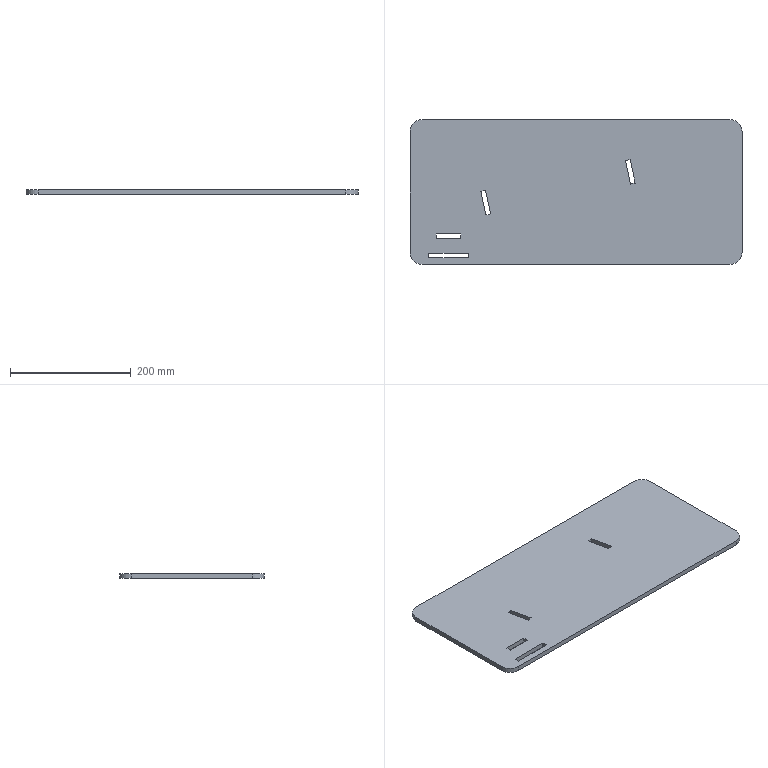Part | SolidWorks | features FlatPattern 1, SMBaseFlange 1, SheetMetal 1 | 1 solid | 26 faces | box 550 x 240 x 8 mm | volume 1041413 mm3 | plane 22 | cylinder 4 | commonest cylinder face diameters 40 x4
STEP:
#1=CARTESIAN_POINT('',(-185.,180.,0.));
#2=VERTEX_POINT('',#1);
#3=CARTESIAN_POINT('',(-205.,160.,0.));
#4=VERTEX_POINT('',#3);
#5=CARTESIAN_POINT('',(-185.,160.,0.));
#6=DIRECTION('',(0.,0.,1.));
#7=DIRECTION('',(1.,0.,0.));
#8=AXIS2_PLACEMENT_3D('',#5,#6,#7);
#9=CIRCLE('',#8,20.);
#10=EDGE_CURVE('',#2,#4,#9,.T.);
#11=ORIENTED_EDGE('',*,*,#10,.F.);
#12=CARTESIAN_POINT('',(-185.,180.,-8.));
#13=VERTEX_POINT('',#12);
#14=CARTESIAN_POINT('',(-185.,180.,-8.));
#15=DIRECTION('',(0.,0.,1.));
#16=VECTOR('',#15,1000.);
#17=LINE('',#14,#16);
#18=EDGE_CURVE('',#13,#2,#17,.T.);
#19=ORIENTED_EDGE('',*,*,#18,.F.);
#20=CARTESIAN_POINT('',(-205.,160.,-8.));
#21=VERTEX_POINT('',#20);
#22=CARTESIAN_POINT('',(-185.,160.,-8.));
#23=DIRECTION('',(0.,0.,1.));
#24=DIRECTION('',(1.,0.,0.));
#25=AXIS2_PLACEMENT_3D('',#22,#23,#24);
#26=CIRCLE('',#25,20.);
#27=EDGE_CURVE('',#13,#21,#26,.T.);
#28=ORIENTED_EDGE('',*,*,#27,.T.);
#29=CARTESIAN_POINT('',(-205.,160.,-8.));
#30=DIRECTION('',(0.,0.,1.));
#31=VECTOR('',#30,1000.);
#32=LINE('',#29,#31);
#33=EDGE_CURVE('',#21,#4,#32,.T.);
#34=ORIENTED_EDGE('',*,*,#33,.T.);
#35=EDGE_LOOP('',(#11,#19,#28,#34));
#36=FACE_OUTER_BOUND('',#35,.T.);
#37=CARTESIAN_POINT('',(-185.,160.,-8.));
#38=DIRECTION('',(0.,0.,1.));
#39=DIRECTION('',(1.,0.,0.));
#40=AXIS2_PLACEMENT_3D('',#37,#38,#39);
#41=CYLINDRICAL_SURFACE('',#40,20.);
#42=ADVANCED_FACE('',(#36),#41,.T.);
#43=CARTESIAN_POINT('',(325.,180.,0.));
#44=VERTEX_POINT('',#43);
#45=CARTESIAN_POINT('',(325.,180.,0.));
#46=DIRECTION('',(-1.,0.,0.));
#47=VECTOR('',#46,1000.);
#48=LINE('',#45,#47);
#49=EDGE_CURVE('',#44,#2,#48,.T.);
#50=ORIENTED_EDGE('',*,*,#49,.F.);
#51=CARTESIAN_POINT('',(325.,180.,-8.));
#52=VERTEX_POINT('',#51);
#53=CARTESIAN_POINT('',(325.,180.,-8.));
#54=DIRECTION('',(0.,0.,1.));
#55=VECTOR('',#54,1000.);
#56=LINE('',#53,#55);
#57=EDGE_CURVE('',#52,#44,#56,.T.);
#58=ORIENTED_EDGE('',*,*,#57,.F.);
#59=CARTESIAN_POINT('',(325.,180.,-8.));
#60=DIRECTION('',(-1.,0.,0.));
#61=VECTOR('',#60,1000.);
#62=LINE('',#59,#61);
#63=EDGE_CURVE('',#52,#13,#62,.T.);
#64=ORIENTED_EDGE('',*,*,#63,.T.);
#65=ORIENTED_EDGE('',*,*,#18,.T.);
#66=EDGE_LOOP('',(#50,#58,#64,#65));
#67=FACE_OUTER_BOUND('',#66,.T.);
#68=CARTESIAN_POINT('',(325.,180.,-8.));
#69=DIRECTION('',(0.,1.,0.));
#70=DIRECTION('',(-1.,0.,0.));
#71=AXIS2_PLACEMENT_3D('',#68,#69,#70);
#72=PLANE('',#71);
#73=ADVANCED_FACE('',(#67),#72,.T.);
#74=CARTESIAN_POINT('',(345.,160.,0.));
#75=VERTEX_POINT('',#74);
#76=CARTESIAN_POINT('',(325.,160.,0.));
#77=DIRECTION('',(0.,0.,1.));
#78=DIRECTION('',(1.,0.,0.));
#79=AXIS2_PLACEMENT_3D('',#76,#77,#78);
#80=CIRCLE('',#79,20.);
#81=EDGE_CURVE('',#75,#44,#80,.T.);
#82=ORIENTED_EDGE('',*,*,#81,.F.);
#83=CARTESIAN_POINT('',(345.,160.,-8.));
#84=VERTEX_POINT('',#83);
#85=CARTESIAN_POINT('',(345.,160.,-8.));
#86=DIRECTION('',(0.,0.,1.));
#87=VECTOR('',#86,1000.);
#88=LINE('',#85,#87);
#89=EDGE_CURVE('',#84,#75,#88,.T.);
#90=ORIENTED_EDGE('',*,*,#89,.F.);
#91=CARTESIAN_POINT('',(325.,160.,-8.));
#92=DIRECTION('',(0.,0.,1.));
#93=DIRECTION('',(1.,0.,0.));
#94=AXIS2_PLACEMENT_3D('',#91,#92,#93);
#95=CIRCLE('',#94,20.);
#96=EDGE_CURVE('',#84,#52,#95,.T.);
#97=ORIENTED_EDGE('',*,*,#96,.T.);
#98=ORIENTED_EDGE('',*,*,#57,.T.);
#99=EDGE_LOOP('',(#82,#90,#97,#98));
#100=FACE_OUTER_BOUND('',#99,.T.);
#101=CARTESIAN_POINT('',(325.,160.,-8.));
#102=DIRECTION('',(0.,0.,1.));
#103=DIRECTION('',(1.,0.,0.));
#104=AXIS2_PLACEMENT_3D('',#101,#102,#103);
#105=CYLINDRICAL_SURFACE('',#104,20.);
#106=ADVANCED_FACE('',(#100),#105,.T.);
#107=CARTESIAN_POINT('',(345.,-40.,0.));
#108=VERTEX_POINT('',#107);
#109=CARTESIAN_POINT('',(345.,160.,0.));
#110=DIRECTION('',(0.,1.,0.));
#111=VECTOR('',#110,1000.);
#112=LINE('',#109,#111);
#113=EDGE_CURVE('',#108,#75,#112,.T.);
#114=ORIENTED_EDGE('',*,*,#113,.F.);
#115=CARTESIAN_POINT('',(345.,-40.,-8.));
#116=VERTEX_POINT('',#115);
#117=CARTESIAN_POINT('',(345.,-40.,-8.));
#118=DIRECTION('',(0.,0.,1.));
#119=VECTOR('',#118,1000.);
#120=LINE('',#117,#119);
#121=EDGE_CURVE('',#116,#108,#120,.T.);
#122=ORIENTED_EDGE('',*,*,#121,.F.);
#123=CARTESIAN_POINT('',(345.,160.,-8.));
#124=DIRECTION('',(0.,1.,0.));
#125=VECTOR('',#124,1000.);
#126=LINE('',#123,#125);
#127=EDGE_CURVE('',#116,#84,#126,.T.);
#128=ORIENTED_EDGE('',*,*,#127,.T.);
#129=ORIENTED_EDGE('',*,*,#89,.T.);
#130=EDGE_LOOP('',(#114,#122,#128,#129));
#131=FACE_OUTER_BOUND('',#130,.T.);
#132=CARTESIAN_POINT('',(345.,160.,-8.));
#133=DIRECTION('',(1.,0.,0.));
#134=DIRECTION('',(0.,1.,0.));
#135=AXIS2_PLACEMENT_3D('',#132,#133,#134);
#136=PLANE('',#135);
#137=ADVANCED_FACE('',(#131),#136,.T.);
#138=CARTESIAN_POINT('',(325.,-60.,0.));
#139=VERTEX_POINT('',#138);
#140=CARTESIAN_POINT('',(325.,-40.,0.));
#141=DIRECTION('',(0.,0.,1.));
#142=DIRECTION('',(1.,0.,0.));
#143=AXIS2_PLACEMENT_3D('',#140,#141,#142);
#144=CIRCLE('',#143,20.);
#145=EDGE_CURVE('',#139,#108,#144,.T.);
#146=ORIENTED_EDGE('',*,*,#145,.F.);
#147=CARTESIAN_POINT('',(325.,-60.,-8.));
#148=VERTEX_POINT('',#147);
#149=CARTESIAN_POINT('',(325.,-60.,-8.));
#150=DIRECTION('',(0.,0.,1.));
#151=VECTOR('',#150,1000.);
#152=LINE('',#149,#151);
#153=EDGE_CURVE('',#148,#139,#152,.T.);
#154=ORIENTED_EDGE('',*,*,#153,.F.);
#155=CARTESIAN_POINT('',(325.,-40.,-8.));
#156=DIRECTION('',(0.,0.,1.));
#157=DIRECTION('',(1.,0.,0.));
#158=AXIS2_PLACEMENT_3D('',#155,#156,#157);
#159=CIRCLE('',#158,20.);
#160=EDGE_CURVE('',#148,#116,#159,.T.);
#161=ORIENTED_EDGE('',*,*,#160,.T.);
#162=ORIENTED_EDGE('',*,*,#121,.T.);
#163=EDGE_LOOP('',(#146,#154,#161,#162));
#164=FACE_OUTER_BOUND('',#163,.T.);
#165=CARTESIAN_POINT('',(325.,-40.,-8.));
#166=DIRECTION('',(0.,0.,1.));
#167=DIRECTION('',(1.,0.,0.));
#168=AXIS2_PLACEMENT_3D('',#165,#166,#167);
#169=CYLINDRICAL_SURFACE('',#168,20.);
#170=ADVANCED_FACE('',(#164),#169,.T.);
#171=CARTESIAN_POINT('',(-185.,-60.,0.));
#172=VERTEX_POINT('',#171);
#173=CARTESIAN_POINT('',(-185.,-60.,0.));
#174=DIRECTION('',(1.,0.,0.));
#175=VECTOR('',#174,1000.);
#176=LINE('',#173,#175);
#177=EDGE_CURVE('',#172,#139,#176,.T.);
#178=ORIENTED_EDGE('',*,*,#177,.F.);
#179=CARTESIAN_POINT('',(-185.,-60.,-8.));
#180=VERTEX_POINT('',#179);
#181=CARTESIAN_POINT('',(-185.,-60.,-8.));
#182=DIRECTION('',(0.,0.,1.));
#183=VECTOR('',#182,1000.);
#184=LINE('',#181,#183);
#185=EDGE_CURVE('',#180,#172,#184,.T.);
#186=ORIENTED_EDGE('',*,*,#185,.F.);
#187=CARTESIAN_POINT('',(-185.,-60.,-8.));
#188=DIRECTION('',(1.,0.,0.));
#189=VECTOR('',#188,1000.);
#190=LINE('',#187,#189);
#191=EDGE_CURVE('',#180,#148,#190,.T.);
#192=ORIENTED_EDGE('',*,*,#191,.T.);
#193=ORIENTED_EDGE('',*,*,#153,.T.);
#194=EDGE_LOOP('',(#178,#186,#192,#193));
#195=FACE_OUTER_BOUND('',#194,.T.);
#196=CARTESIAN_POINT('',(-185.,-60.,-8.));
#197=DIRECTION('',(0.,-1.,0.));
#198=DIRECTION('',(0.,0.,-1.));
#199=AXIS2_PLACEMENT_3D('',#196,#197,#198);
#200=PLANE('',#199);
#201=ADVANCED_FACE('',(#195),#200,.T.);
#202=CARTESIAN_POINT('',(-205.,-40.,0.));
#203=VERTEX_POINT('',#202);
#204=CARTESIAN_POINT('',(-185.,-40.,0.));
#205=DIRECTION('',(0.,0.,1.));
#206=DIRECTION('',(-1.,0.,0.));
#207=AXIS2_PLACEMENT_3D('',#204,#205,#206);
#208=CIRCLE('',#207,20.);
#209=EDGE_CURVE('',#203,#172,#208,.T.);
#210=ORIENTED_EDGE('',*,*,#209,.F.);
#211=CARTESIAN_POINT('',(-205.,-40.,-8.));
#212=VERTEX_POINT('',#211);
#213=CARTESIAN_POINT('',(-205.,-40.,-8.));
#214=DIRECTION('',(0.,0.,1.));
#215=VECTOR('',#214,1000.);
#216=LINE('',#213,#215);
#217=EDGE_CURVE('',#212,#203,#216,.T.);
#218=ORIENTED_EDGE('',*,*,#217,.F.);
#219=CARTESIAN_POINT('',(-185.,-40.,-8.));
#220=DIRECTION('',(0.,0.,1.));
#221=DIRECTION('',(-1.,0.,0.));
#222=AXIS2_PLACEMENT_3D('',#219,#220,#221);
#223=CIRCLE('',#222,20.);
#224=EDGE_CURVE('',#212,#180,#223,.T.);
#225=ORIENTED_EDGE('',*,*,#224,.T.);
#226=ORIENTED_EDGE('',*,*,#185,.T.);
#227=EDGE_LOOP('',(#210,#218,#225,#226));
#228=FACE_OUTER_BOUND('',#227,.T.);
#229=CARTESIAN_POINT('',(-185.,-40.,-8.));
#230=DIRECTION('',(0.,0.,1.));
#231=DIRECTION('',(1.,0.,0.));
#232=AXIS2_PLACEMENT_3D('',#229,#230,#231);
#233=CYLINDRICAL_SURFACE('',#232,20.);
#234=ADVANCED_FACE('',(#228),#233,.T.);
#235=CARTESIAN_POINT('',(-205.,160.,0.));
#236=DIRECTION('',(0.,-1.,0.));
#237=VECTOR('',#236,1000.);
#238=LINE('',#235,#237);
#239=EDGE_CURVE('',#4,#203,#238,.T.);
#240=ORIENTED_EDGE('',*,*,#239,.F.);
#241=ORIENTED_EDGE('',*,*,#33,.F.);
#242=CARTESIAN_POINT('',(-205.,160.,-8.));
#243=DIRECTION('',(0.,-1.,0.));
#244=VECTOR('',#243,1000.);
#245=LINE('',#242,#244);
#246=EDGE_CURVE('',#21,#212,#245,.T.);
#247=ORIENTED_EDGE('',*,*,#246,.T.);
#248=ORIENTED_EDGE('',*,*,#217,.T.);
#249=EDGE_LOOP('',(#240,#241,#247,#248));
#250=FACE_OUTER_BOUND('',#249,.T.);
#251=CARTESIAN_POINT('',(-205.,160.,-8.));
#252=DIRECTION('',(-1.,0.,0.));
#253=DIRECTION('',(0.,-1.,0.));
#254=AXIS2_PLACEMENT_3D('',#251,#252,#253);
#255=PLANE('',#254);
#256=ADVANCED_FACE('',(#250),#255,.T.);
#257=CARTESIAN_POINT('',(-121.165,-9.311,-8.));
#258=VERTEX_POINT('',#257);
#259=CARTESIAN_POINT('',(-161.165,-9.311,-8.));
#260=VERTEX_POINT('',#259);
#261=CARTESIAN_POINT('',(-161.165,-9.311,-8.));
#262=DIRECTION('',(-1.,0.,0.));
#263=VECTOR('',#262,1000.);
#264=LINE('',#261,#263);
#265=EDGE_CURVE('',#258,#260,#264,.T.);
#266=ORIENTED_EDGE('',*,*,#265,.T.);
#267=CARTESIAN_POINT('',(-161.165,-17.311,-8.));
#268=VERTEX_POINT('',#267);
#269=CARTESIAN_POINT('',(-161.165,-9.311,-8.));
#270=DIRECTION('',(0.,-1.,0.));
#271=VECTOR('',#270,1000.);
#272=LINE('',#269,#271);
#273=EDGE_CURVE('',#260,#268,#272,.T.);
#274=ORIENTED_EDGE('',*,*,#273,.T.);
#275=CARTESIAN_POINT('',(-121.165,-17.311,-8.));
#276=VERTEX_POINT('',#275);
#277=CARTESIAN_POINT('',(-161.165,-17.311,-8.));
#278=DIRECTION('',(1.,0.,0.));
#279=VECTOR('',#278,1000.);
#280=LINE('',#277,#279);
#281=EDGE_CURVE('',#268,#276,#280,.T.);
#282=ORIENTED_EDGE('',*,*,#281,.T.);
#283=CARTESIAN_POINT('',(-121.165,-9.311,-8.));
#284=DIRECTION('',(0.,1.,0.));
#285=VECTOR('',#284,1000.);
#286=LINE('',#283,#285);
#287=EDGE_CURVE('',#276,#258,#286,.T.);
#288=ORIENTED_EDGE('',*,*,#287,.T.);
#289=EDGE_LOOP('',(#266,#274,#282,#288));
#290=FACE_BOUND('',#289,.T.);
#291=CARTESIAN_POINT('',(159.735,113.821,-8.));
#292=VERTEX_POINT('',#291);
#293=CARTESIAN_POINT('',(151.91,112.158,-8.));
#294=VERTEX_POINT('',#293);
#295=CARTESIAN_POINT('',(151.91,112.158,-8.));
#296=DIRECTION('',(-0.9781,-0.2079,0.));
#297=VECTOR('',#296,1000.);
#298=LINE('',#295,#297);
#299=EDGE_CURVE('',#292,#294,#298,.T.);
#300=ORIENTED_EDGE('',*,*,#299,.T.);
#301=CARTESIAN_POINT('',(160.226,73.032,-8.));
#302=VERTEX_POINT('',#301);
#303=CARTESIAN_POINT('',(160.226,73.032,-8.));
#304=DIRECTION('',(0.2079,-0.9781,0.));
#305=VECTOR('',#304,1000.);
#306=LINE('',#303,#305);
#307=EDGE_CURVE('',#294,#302,#306,.T.);
#308=ORIENTED_EDGE('',*,*,#307,.T.);
#309=CARTESIAN_POINT('',(168.051,74.695,-8.));
#310=VERTEX_POINT('',#309);
#311=CARTESIAN_POINT('',(168.051,74.695,-8.));
#312=DIRECTION('',(0.9781,0.2079,0.));
#313=VECTOR('',#312,1000.);
#314=LINE('',#311,#313);
#315=EDGE_CURVE('',#302,#310,#314,.T.);
#316=ORIENTED_EDGE('',*,*,#315,.T.);
#317=CARTESIAN_POINT('',(159.735,113.821,-8.));
#318=DIRECTION('',(-0.2079,0.9781,0.));
#319=VECTOR('',#318,1000.);
#320=LINE('',#317,#319);
#321=EDGE_CURVE('',#310,#292,#320,.T.);
#322=ORIENTED_EDGE('',*,*,#321,.T.);
#323=EDGE_LOOP('',(#300,#308,#316,#322));
#324=FACE_BOUND('',#323,.T.);
#325=CARTESIAN_POINT('',(-108.665,-41.311,-8.));
#326=VERTEX_POINT('',#325);
#327=CARTESIAN_POINT('',(-173.665,-41.311,-8.));
#328=VERTEX_POINT('',#327);
#329=CARTESIAN_POINT('',(-173.665,-41.311,-8.));
#330=DIRECTION('',(-1.,0.,0.));
#331=VECTOR('',#330,1000.);
#332=LINE('',#329,#331);
#333=EDGE_CURVE('',#326,#328,#332,.T.);
#334=ORIENTED_EDGE('',*,*,#333,.T.);
#335=CARTESIAN_POINT('',(-173.665,-49.311,-8.));
#336=VERTEX_POINT('',#335);
#337=CARTESIAN_POINT('',(-173.665,-49.311,-8.));
#338=DIRECTION('',(0.,-1.,0.));
#339=VECTOR('',#338,1000.);
#340=LINE('',#337,#339);
#341=EDGE_CURVE('',#328,#336,#340,.T.);
#342=ORIENTED_EDGE('',*,*,#341,.T.);
#343=CARTESIAN_POINT('',(-108.665,-49.311,-8.));
#344=VERTEX_POINT('',#343);
#345=CARTESIAN_POINT('',(-173.665,-49.311,-8.));
#346=DIRECTION('',(1.,0.,0.));
#347=VECTOR('',#346,1000.);
#348=LINE('',#345,#347);
#349=EDGE_CURVE('',#336,#344,#348,.T.);
#350=ORIENTED_EDGE('',*,*,#349,.T.);
#351=CARTESIAN_POINT('',(-108.665,-49.311,-8.));
#352=DIRECTION('',(0.,1.,0.));
#353=VECTOR('',#352,1000.);
#354=LINE('',#351,#353);
#355=EDGE_CURVE('',#344,#326,#354,.T.);
#356=ORIENTED_EDGE('',*,*,#355,.T.);
#357=EDGE_LOOP('',(#334,#342,#350,#356));
#358=FACE_BOUND('',#357,.T.);
#359=CARTESIAN_POINT('',(-79.911,62.882,-8.));
#360=VERTEX_POINT('',#359);
#361=CARTESIAN_POINT('',(-87.737,61.219,-8.));
#362=VERTEX_POINT('',#361);
#363=CARTESIAN_POINT('',(-87.737,61.219,-8.));
#364=DIRECTION('',(-0.9781,-0.2079,0.));
#365=VECTOR('',#364,1000.);
#366=LINE('',#363,#365);
#367=EDGE_CURVE('',#360,#362,#366,.T.);
#368=ORIENTED_EDGE('',*,*,#367,.T.);
#369=CARTESIAN_POINT('',(-79.42,22.093,-8.));
#370=VERTEX_POINT('',#369);
#371=CARTESIAN_POINT('',(-79.42,22.093,-8.));
#372=DIRECTION('',(0.2079,-0.9781,0.));
#373=VECTOR('',#372,1000.);
#374=LINE('',#371,#373);
#375=EDGE_CURVE('',#362,#370,#374,.T.);
#376=ORIENTED_EDGE('',*,*,#375,.T.);
#377=CARTESIAN_POINT('',(-71.595,23.757,-8.));
#378=VERTEX_POINT('',#377);
#379=CARTESIAN_POINT('',(-71.595,23.757,-8.));
#380=DIRECTION('',(0.9781,0.2079,0.));
#381=VECTOR('',#380,1000.);
#382=LINE('',#379,#381);
#383=EDGE_CURVE('',#370,#378,#382,.T.);
#384=ORIENTED_EDGE('',*,*,#383,.T.);
#385=CARTESIAN_POINT('',(-79.911,62.882,-8.));
#386=DIRECTION('',(-0.2079,0.9781,0.));
#387=VECTOR('',#386,1000.);
#388=LINE('',#385,#387);
#389=EDGE_CURVE('',#378,#360,#388,.T.);
#390=ORIENTED_EDGE('',*,*,#389,.T.);
#391=EDGE_LOOP('',(#368,#376,#384,#390));
#392=FACE_BOUND('',#391,.T.);
#393=ORIENTED_EDGE('',*,*,#27,.F.);
#394=ORIENTED_EDGE('',*,*,#63,.F.);
#395=ORIENTED_EDGE('',*,*,#96,.F.);
#396=ORIENTED_EDGE('',*,*,#127,.F.);
#397=ORIENTED_EDGE('',*,*,#160,.F.);
#398=ORIENTED_EDGE('',*,*,#191,.F.);
#399=ORIENTED_EDGE('',*,*,#224,.F.);
#400=ORIENTED_EDGE('',*,*,#246,.F.);
#401=EDGE_LOOP('',(#393,#394,#395,#396,#397,#398,#399,#400));
#402=FACE_OUTER_BOUND('',#401,.T.);
#403=CARTESIAN_POINT('',(-185.,160.,-8.));
#404=DIRECTION('',(0.,0.,1.));
#405=DIRECTION('',(1.,0.,0.));
#406=AXIS2_PLACEMENT_3D('',#403,#404,#405);
#407=PLANE('',#406);
#408=ADVANCED_FACE('',(#290,#324,#358,#392,#402),#407,.F.);
#409=CARTESIAN_POINT('',(-161.165,-9.311,0.));
#410=VERTEX_POINT('',#409);
#411=CARTESIAN_POINT('',(-161.165,-17.311,0.));
#412=VERTEX_POINT('',#411);
#413=CARTESIAN_POINT('',(-161.165,-9.311,0.));
#414=DIRECTION('',(0.,-1.,0.));
#415=VECTOR('',#414,1000.);
#416=LINE('',#413,#415);
#417=EDGE_CURVE('',#410,#412,#416,.T.);
#418=ORIENTED_EDGE('',*,*,#417,.F.);
#419=CARTESIAN_POINT('',(-121.165,-9.311,0.));
#420=VERTEX_POINT('',#419);
#421=CARTESIAN_POINT('',(-161.165,-9.311,0.));
#422=DIRECTION('',(-1.,0.,0.));
#423=VECTOR('',#422,1000.);
#424=LINE('',#421,#423);
#425=EDGE_CURVE('',#420,#410,#424,.T.);
#426=ORIENTED_EDGE('',*,*,#425,.F.);
#427=CARTESIAN_POINT('',(-121.165,-17.311,0.));
#428=VERTEX_POINT('',#427);
#429=CARTESIAN_POINT('',(-121.165,-9.311,0.));
#430=DIRECTION('',(0.,1.,0.));
#431=VECTOR('',#430,1000.);
#432=LINE('',#429,#431);
#433=EDGE_CURVE('',#428,#420,#432,.T.);
#434=ORIENTED_EDGE('',*,*,#433,.F.);
#435=CARTESIAN_POINT('',(-161.165,-17.311,0.));
#436=DIRECTION('',(1.,0.,0.));
#437=VECTOR('',#436,1000.);
#438=LINE('',#435,#437);
#439=EDGE_CURVE('',#412,#428,#438,.T.);
#440=ORIENTED_EDGE('',*,*,#439,.F.);
#441=EDGE_LOOP('',(#418,#426,#434,#440));
#442=FACE_BOUND('',#441,.T.);
#443=CARTESIAN_POINT('',(151.91,112.158,0.));
#444=VERTEX_POINT('',#443);
#445=CARTESIAN_POINT('',(160.226,73.032,0.));
#446=VERTEX_POINT('',#445);
#447=CARTESIAN_POINT('',(160.226,73.032,0.));
#448=DIRECTION('',(0.2079,-0.9781,0.));
#449=VECTOR('',#448,1000.);
#450=LINE('',#447,#449);
#451=EDGE_CURVE('',#444,#446,#450,.T.);
#452=ORIENTED_EDGE('',*,*,#451,.F.);
#453=CARTESIAN_POINT('',(159.735,113.821,0.));
#454=VERTEX_POINT('',#453);
#455=CARTESIAN_POINT('',(151.91,112.158,0.));
#456=DIRECTION('',(-0.9781,-0.2079,0.));
#457=VECTOR('',#456,1000.);
#458=LINE('',#455,#457);
#459=EDGE_CURVE('',#454,#444,#458,.T.);
#460=ORIENTED_EDGE('',*,*,#459,.F.);
#461=CARTESIAN_POINT('',(168.051,74.695,0.));
#462=VERTEX_POINT('',#461);
#463=CARTESIAN_POINT('',(159.735,113.821,0.));
#464=DIRECTION('',(-0.2079,0.9781,0.));
#465=VECTOR('',#464,1000.);
#466=LINE('',#463,#465);
#467=EDGE_CURVE('',#462,#454,#466,.T.);
#468=ORIENTED_EDGE('',*,*,#467,.F.);
#469=CARTESIAN_POINT('',(168.051,74.695,0.));
#470=DIRECTION('',(0.9781,0.2079,0.));
#471=VECTOR('',#470,1000.);
#472=LINE('',#469,#471);
#473=EDGE_CURVE('',#446,#462,#472,.T.);
#474=ORIENTED_EDGE('',*,*,#473,.F.);
#475=EDGE_LOOP('',(#452,#460,#468,#474));
#476=FACE_BOUND('',#475,.T.);
#477=CARTESIAN_POINT('',(-173.665,-41.311,0.));
#478=VERTEX_POINT('',#477);
#479=CARTESIAN_POINT('',(-173.665,-49.311,0.));
#480=VERTEX_POINT('',#479);
#481=CARTESIAN_POINT('',(-173.665,-49.311,0.));
#482=DIRECTION('',(0.,-1.,0.));
#483=VECTOR('',#482,1000.);
#484=LINE('',#481,#483);
#485=EDGE_CURVE('',#478,#480,#484,.T.);
#486=ORIENTED_EDGE('',*,*,#485,.F.);
#487=CARTESIAN_POINT('',(-108.665,-41.311,0.));
#488=VERTEX_POINT('',#487);
#489=CARTESIAN_POINT('',(-173.665,-41.311,0.));
#490=DIRECTION('',(-1.,0.,0.));
#491=VECTOR('',#490,1000.);
#492=LINE('',#489,#491);
#493=EDGE_CURVE('',#488,#478,#492,.T.);
#494=ORIENTED_EDGE('',*,*,#493,.F.);
#495=CARTESIAN_POINT('',(-108.665,-49.311,0.));
#496=VERTEX_POINT('',#495);
#497=CARTESIAN_POINT('',(-108.665,-49.311,0.));
#498=DIRECTION('',(0.,1.,0.));
#499=VECTOR('',#498,1000.);
#500=LINE('',#497,#499);
#501=EDGE_CURVE('',#496,#488,#500,.T.);
#502=ORIENTED_EDGE('',*,*,#501,.F.);
#503=CARTESIAN_POINT('',(-173.665,-49.311,0.));
#504=DIRECTION('',(1.,0.,0.));
#505=VECTOR('',#504,1000.);
#506=LINE('',#503,#505);
#507=EDGE_CURVE('',#480,#496,#506,.T.);
#508=ORIENTED_EDGE('',*,*,#507,.F.);
#509=EDGE_LOOP('',(#486,#494,#502,#508));
#510=FACE_BOUND('',#509,.T.);
#511=CARTESIAN_POINT('',(-87.737,61.219,0.));
#512=VERTEX_POINT('',#511);
#513=CARTESIAN_POINT('',(-79.42,22.093,0.));
#514=VERTEX_POINT('',#513);
#515=CARTESIAN_POINT('',(-79.42,22.093,0.));
#516=DIRECTION('',(0.2079,-0.9781,0.));
#517=VECTOR('',#516,1000.);
#518=LINE('',#515,#517);
#519=EDGE_CURVE('',#512,#514,#518,.T.);
#520=ORIENTED_EDGE('',*,*,#519,.F.);
#521=CARTESIAN_POINT('',(-79.911,62.882,0.));
#522=VERTEX_POINT('',#521);
#523=CARTESIAN_POINT('',(-87.737,61.219,0.));
#524=DIRECTION('',(-0.9781,-0.2079,0.));
#525=VECTOR('',#524,1000.);
#526=LINE('',#523,#525);
#527=EDGE_CURVE('',#522,#512,#526,.T.);
#528=ORIENTED_EDGE('',*,*,#527,.F.);
#529=CARTESIAN_POINT('',(-71.595,23.757,0.));
#530=VERTEX_POINT('',#529);
#531=CARTESIAN_POINT('',(-79.911,62.882,0.));
#532=DIRECTION('',(-0.2079,0.9781,0.));
#533=VECTOR('',#532,1000.);
#534=LINE('',#531,#533);
#535=EDGE_CURVE('',#530,#522,#534,.T.);
#536=ORIENTED_EDGE('',*,*,#535,.F.);
#537=CARTESIAN_POINT('',(-71.595,23.757,0.));
#538=DIRECTION('',(0.9781,0.2079,0.));
#539=VECTOR('',#538,1000.);
#540=LINE('',#537,#539);
#541=EDGE_CURVE('',#514,#530,#540,.T.);
#542=ORIENTED_EDGE('',*,*,#541,.F.);
#543=EDGE_LOOP('',(#520,#528,#536,#542));
#544=FACE_BOUND('',#543,.T.);
#545=ORIENTED_EDGE('',*,*,#10,.T.);
#546=ORIENTED_EDGE('',*,*,#239,.T.);
#547=ORIENTED_EDGE('',*,*,#209,.T.);
#548=ORIENTED_EDGE('',*,*,#177,.T.);
#549=ORIENTED_EDGE('',*,*,#145,.T.);
#550=ORIENTED_EDGE('',*,*,#113,.T.);
#551=ORIENTED_EDGE('',*,*,#81,.T.);
#552=ORIENTED_EDGE('',*,*,#49,.T.);
#553=EDGE_LOOP('',(#545,#546,#547,#548,#549,#550,#551,#552));
#554=FACE_OUTER_BOUND('',#553,.T.);
#555=CARTESIAN_POINT('',(-185.,160.,0.));
#556=DIRECTION('',(0.,0.,1.));
#557=DIRECTION('',(1.,0.,0.));
#558=AXIS2_PLACEMENT_3D('',#555,#556,#557);
#559=PLANE('',#558);
#560=ADVANCED_FACE('',(#442,#476,#510,#544,#554),#559,.T.);
#561=ORIENTED_EDGE('',*,*,#519,.T.);
#562=CARTESIAN_POINT('',(-79.42,22.093,-8.));
#563=DIRECTION('',(0.,0.,1.));
#564=VECTOR('',#563,1000.);
#565=LINE('',#562,#564);
#566=EDGE_CURVE('',#370,#514,#565,.T.);
#567=ORIENTED_EDGE('',*,*,#566,.F.);
#568=ORIENTED_EDGE('',*,*,#375,.F.);
#569=CARTESIAN_POINT('',(-87.737,61.219,-8.));
#570=DIRECTION('',(0.,0.,1.));
#571=VECTOR('',#570,1000.);
#572=LINE('',#569,#571);
#573=EDGE_CURVE('',#362,#512,#572,.T.);
#574=ORIENTED_EDGE('',*,*,#573,.T.);
#575=EDGE_LOOP('',(#561,#567,#568,#574));
#576=FACE_OUTER_BOUND('',#575,.T.);
#577=CARTESIAN_POINT('',(-79.42,22.093,-8.));
#578=DIRECTION('',(-0.9781,-0.2079,0.));
#579=DIRECTION('',(0.2079,-0.9781,0.));
#580=AXIS2_PLACEMENT_3D('',#577,#578,#579);
#581=PLANE('',#580);
#582=ADVANCED_FACE('',(#576),#581,.F.);
#583=ORIENTED_EDGE('',*,*,#527,.T.);
#584=ORIENTED_EDGE('',*,*,#573,.F.);
#585=ORIENTED_EDGE('',*,*,#367,.F.);
#586=CARTESIAN_POINT('',(-79.911,62.882,-8.));
#587=DIRECTION('',(0.,0.,1.));
#588=VECTOR('',#587,1000.);
#589=LINE('',#586,#588);
#590=EDGE_CURVE('',#360,#522,#589,.T.);
#591=ORIENTED_EDGE('',*,*,#590,.T.);
#592=EDGE_LOOP('',(#583,#584,#585,#591));
#593=FACE_OUTER_BOUND('',#592,.T.);
#594=CARTESIAN_POINT('',(-87.737,61.219,-8.));
#595=DIRECTION('',(-0.2079,0.9781,0.));
#596=DIRECTION('',(-0.9781,-0.2079,0.));
#597=AXIS2_PLACEMENT_3D('',#594,#595,#596);
#598=PLANE('',#597);
#599=ADVANCED_FACE('',(#593),#598,.F.);
#600=ORIENTED_EDGE('',*,*,#535,.T.);
#601=ORIENTED_EDGE('',*,*,#590,.F.);
#602=ORIENTED_EDGE('',*,*,#389,.F.);
#603=CARTESIAN_POINT('',(-71.595,23.757,-8.));
#604=DIRECTION('',(0.,0.,1.));
#605=VECTOR('',#604,1000.);
#606=LINE('',#603,#605);
#607=EDGE_CURVE('',#378,#530,#606,.T.);
#608=ORIENTED_EDGE('',*,*,#607,.T.);
#609=EDGE_LOOP('',(#600,#601,#602,#608));
#610=FACE_OUTER_BOUND('',#609,.T.);
#611=CARTESIAN_POINT('',(-79.911,62.882,-8.));
#612=DIRECTION('',(0.9781,0.2079,0.));
#613=DIRECTION('',(-0.2079,0.9781,0.));
#614=AXIS2_PLACEMENT_3D('',#611,#612,#613);
#615=PLANE('',#614);
#616=ADVANCED_FACE('',(#610),#615,.F.);
#617=ORIENTED_EDGE('',*,*,#541,.T.);
#618=ORIENTED_EDGE('',*,*,#607,.F.);
#619=ORIENTED_EDGE('',*,*,#383,.F.);
#620=ORIENTED_EDGE('',*,*,#566,.T.);
#621=EDGE_LOOP('',(#617,#618,#619,#620));
#622=FACE_OUTER_BOUND('',#621,.T.);
#623=CARTESIAN_POINT('',(-71.595,23.757,-8.));
#624=DIRECTION('',(0.2079,-0.9781,0.));
#625=DIRECTION('',(0.9781,0.2079,0.));
#626=AXIS2_PLACEMENT_3D('',#623,#624,#625);
#627=PLANE('',#626);
#628=ADVANCED_FACE('',(#622),#627,.F.);
#629=ORIENTED_EDGE('',*,*,#485,.T.);
#630=CARTESIAN_POINT('',(-173.665,-49.311,-8.));
#631=DIRECTION('',(0.,0.,1.));
#632=VECTOR('',#631,1000.);
#633=LINE('',#630,#632);
#634=EDGE_CURVE('',#336,#480,#633,.T.);
#635=ORIENTED_EDGE('',*,*,#634,.F.);
#636=ORIENTED_EDGE('',*,*,#341,.F.);
#637=CARTESIAN_POINT('',(-173.665,-41.311,-8.));
#638=DIRECTION('',(0.,0.,1.));
#639=VECTOR('',#638,1000.);
#640=LINE('',#637,#639);
#641=EDGE_CURVE('',#328,#478,#640,.T.);
#642=ORIENTED_EDGE('',*,*,#641,.T.);
#643=EDGE_LOOP('',(#629,#635,#636,#642));
#644=FACE_OUTER_BOUND('',#643,.T.);
#645=CARTESIAN_POINT('',(-173.665,-49.311,-8.));
#646=DIRECTION('',(-1.,0.,0.));
#647=DIRECTION('',(0.,0.,1.));
#648=AXIS2_PLACEMENT_3D('',#645,#646,#647);
#649=PLANE('',#648);
#650=ADVANCED_FACE('',(#644),#649,.F.);
#651=ORIENTED_EDGE('',*,*,#493,.T.);
#652=ORIENTED_EDGE('',*,*,#641,.F.);
#653=ORIENTED_EDGE('',*,*,#333,.F.);
#654=CARTESIAN_POINT('',(-108.665,-41.311,-8.));
#655=DIRECTION('',(0.,0.,1.));
#656=VECTOR('',#655,1000.);
#657=LINE('',#654,#656);
#658=EDGE_CURVE('',#326,#488,#657,.T.);
#659=ORIENTED_EDGE('',*,*,#658,.T.);
#660=EDGE_LOOP('',(#651,#652,#653,#659));
#661=FACE_OUTER_BOUND('',#660,.T.);
#662=CARTESIAN_POINT('',(-173.665,-41.311,-8.));
#663=DIRECTION('',(0.,1.,0.));
#664=DIRECTION('',(0.,0.,1.));
#665=AXIS2_PLACEMENT_3D('',#662,#663,#664);
#666=PLANE('',#665);
#667=ADVANCED_FACE('',(#661),#666,.F.);
#668=ORIENTED_EDGE('',*,*,#501,.T.);
#669=ORIENTED_EDGE('',*,*,#658,.F.);
#670=ORIENTED_EDGE('',*,*,#355,.F.);
#671=CARTESIAN_POINT('',(-108.665,-49.311,-8.));
#672=DIRECTION('',(0.,0.,1.));
#673=VECTOR('',#672,1000.);
#674=LINE('',#671,#673);
#675=EDGE_CURVE('',#344,#496,#674,.T.);
#676=ORIENTED_EDGE('',*,*,#675,.T.);
#677=EDGE_LOOP('',(#668,#669,#670,#676));
#678=FACE_OUTER_BOUND('',#677,.T.);
#679=CARTESIAN_POINT('',(-108.665,-49.311,-8.));
#680=DIRECTION('',(1.,0.,0.));
#681=DIRECTION('',(0.,0.,-1.));
#682=AXIS2_PLACEMENT_3D('',#679,#680,#681);
#683=PLANE('',#682);
#684=ADVANCED_FACE('',(#678),#683,.F.);
#685=ORIENTED_EDGE('',*,*,#507,.T.);
#686=ORIENTED_EDGE('',*,*,#675,.F.);
#687=ORIENTED_EDGE('',*,*,#349,.F.);
#688=ORIENTED_EDGE('',*,*,#634,.T.);
#689=EDGE_LOOP('',(#685,#686,#687,#688));
#690=FACE_OUTER_BOUND('',#689,.T.);
#691=CARTESIAN_POINT('',(-173.665,-49.311,-8.));
#692=DIRECTION('',(0.,-1.,0.));
#693=DIRECTION('',(0.,0.,-1.));
#694=AXIS2_PLACEMENT_3D('',#691,#692,#693);
#695=PLANE('',#694);
#696=ADVANCED_FACE('',(#690),#695,.F.);
#697=ORIENTED_EDGE('',*,*,#451,.T.);
#698=CARTESIAN_POINT('',(160.226,73.032,-8.));
#699=DIRECTION('',(0.,0.,1.));
#700=VECTOR('',#699,1000.);
#701=LINE('',#698,#700);
#702=EDGE_CURVE('',#302,#446,#701,.T.);
#703=ORIENTED_EDGE('',*,*,#702,.F.);
#704=ORIENTED_EDGE('',*,*,#307,.F.);
#705=CARTESIAN_POINT('',(151.91,112.158,-8.));
#706=DIRECTION('',(0.,0.,1.));
#707=VECTOR('',#706,1000.);
#708=LINE('',#705,#707);
#709=EDGE_CURVE('',#294,#444,#708,.T.);
#710=ORIENTED_EDGE('',*,*,#709,.T.);
#711=EDGE_LOOP('',(#697,#703,#704,#710));
#712=FACE_OUTER_BOUND('',#711,.T.);
#713=CARTESIAN_POINT('',(160.226,73.032,-8.));
#714=DIRECTION('',(-0.9781,-0.2079,0.));
#715=DIRECTION('',(0.2079,-0.9781,0.));
#716=AXIS2_PLACEMENT_3D('',#713,#714,#715);
#717=PLANE('',#716);
#718=ADVANCED_FACE('',(#712),#717,.F.);
#719=ORIENTED_EDGE('',*,*,#459,.T.);
#720=ORIENTED_EDGE('',*,*,#709,.F.);
#721=ORIENTED_EDGE('',*,*,#299,.F.);
#722=CARTESIAN_POINT('',(159.735,113.821,-8.));
#723=DIRECTION('',(0.,0.,1.));
#724=VECTOR('',#723,1000.);
#725=LINE('',#722,#724);
#726=EDGE_CURVE('',#292,#454,#725,.T.);
#727=ORIENTED_EDGE('',*,*,#726,.T.);
#728=EDGE_LOOP('',(#719,#720,#721,#727));
#729=FACE_OUTER_BOUND('',#728,.T.);
#730=CARTESIAN_POINT('',(151.91,112.158,-8.));
#731=DIRECTION('',(-0.2079,0.9781,0.));
#732=DIRECTION('',(-0.9781,-0.2079,0.));
#733=AXIS2_PLACEMENT_3D('',#730,#731,#732);
#734=PLANE('',#733);
#735=ADVANCED_FACE('',(#729),#734,.F.);
#736=ORIENTED_EDGE('',*,*,#467,.T.);
#737=ORIENTED_EDGE('',*,*,#726,.F.);
#738=ORIENTED_EDGE('',*,*,#321,.F.);
#739=CARTESIAN_POINT('',(168.051,74.695,-8.));
#740=DIRECTION('',(0.,0.,1.));
#741=VECTOR('',#740,1000.);
#742=LINE('',#739,#741);
#743=EDGE_CURVE('',#310,#462,#742,.T.);
#744=ORIENTED_EDGE('',*,*,#743,.T.);
#745=EDGE_LOOP('',(#736,#737,#738,#744));
#746=FACE_OUTER_BOUND('',#745,.T.);
#747=CARTESIAN_POINT('',(159.735,113.821,-8.));
#748=DIRECTION('',(0.9781,0.2079,0.));
#749=DIRECTION('',(-0.2079,0.9781,0.));
#750=AXIS2_PLACEMENT_3D('',#747,#748,#749);
#751=PLANE('',#750);
#752=ADVANCED_FACE('',(#746),#751,.F.);
#753=ORIENTED_EDGE('',*,*,#473,.T.);
#754=ORIENTED_EDGE('',*,*,#743,.F.);
#755=ORIENTED_EDGE('',*,*,#315,.F.);
#756=ORIENTED_EDGE('',*,*,#702,.T.);
#757=EDGE_LOOP('',(#753,#754,#755,#756));
#758=FACE_OUTER_BOUND('',#757,.T.);
#759=CARTESIAN_POINT('',(168.051,74.695,-8.));
#760=DIRECTION('',(0.2079,-0.9781,0.));
#761=DIRECTION('',(0.9781,0.2079,0.));
#762=AXIS2_PLACEMENT_3D('',#759,#760,#761);
#763=PLANE('',#762);
#764=ADVANCED_FACE('',(#758),#763,.F.);
#765=ORIENTED_EDGE('',*,*,#417,.T.);
#766=CARTESIAN_POINT('',(-161.165,-17.311,-8.));
#767=DIRECTION('',(0.,0.,1.));
#768=VECTOR('',#767,1000.);
#769=LINE('',#766,#768);
#770=EDGE_CURVE('',#268,#412,#769,.T.);
#771=ORIENTED_EDGE('',*,*,#770,.F.);
#772=ORIENTED_EDGE('',*,*,#273,.F.);
#773=CARTESIAN_POINT('',(-161.165,-9.311,-8.));
#774=DIRECTION('',(0.,0.,1.));
#775=VECTOR('',#774,1000.);
#776=LINE('',#773,#775);
#777=EDGE_CURVE('',#260,#410,#776,.T.);
#778=ORIENTED_EDGE('',*,*,#777,.T.);
#779=EDGE_LOOP('',(#765,#771,#772,#778));
#780=FACE_OUTER_BOUND('',#779,.T.);
#781=CARTESIAN_POINT('',(-161.165,-9.311,-8.));
#782=DIRECTION('',(-1.,0.,0.));
#783=DIRECTION('',(0.,0.,1.));
#784=AXIS2_PLACEMENT_3D('',#781,#782,#783);
#785=PLANE('',#784);
#786=ADVANCED_FACE('',(#780),#785,.F.);
#787=ORIENTED_EDGE('',*,*,#425,.T.);
#788=ORIENTED_EDGE('',*,*,#777,.F.);
#789=ORIENTED_EDGE('',*,*,#265,.F.);
#790=CARTESIAN_POINT('',(-121.165,-9.311,-8.));
#791=DIRECTION('',(0.,0.,1.));
#792=VECTOR('',#791,1000.);
#793=LINE('',#790,#792);
#794=EDGE_CURVE('',#258,#420,#793,.T.);
#795=ORIENTED_EDGE('',*,*,#794,.T.);
#796=EDGE_LOOP('',(#787,#788,#789,#795));
#797=FACE_OUTER_BOUND('',#796,.T.);
#798=CARTESIAN_POINT('',(-161.165,-9.311,-8.));
#799=DIRECTION('',(0.,1.,0.));
#800=DIRECTION('',(0.,0.,1.));
#801=AXIS2_PLACEMENT_3D('',#798,#799,#800);
#802=PLANE('',#801);
#803=ADVANCED_FACE('',(#797),#802,.F.);
#804=ORIENTED_EDGE('',*,*,#433,.T.);
#805=ORIENTED_EDGE('',*,*,#794,.F.);
#806=ORIENTED_EDGE('',*,*,#287,.F.);
#807=CARTESIAN_POINT('',(-121.165,-17.311,-8.));
#808=DIRECTION('',(0.,0.,1.));
#809=VECTOR('',#808,1000.);
#810=LINE('',#807,#809);
#811=EDGE_CURVE('',#276,#428,#810,.T.);
#812=ORIENTED_EDGE('',*,*,#811,.T.);
#813=EDGE_LOOP('',(#804,#805,#806,#812));
#814=FACE_OUTER_BOUND('',#813,.T.);
#815=CARTESIAN_POINT('',(-121.165,-9.311,-8.));
#816=DIRECTION('',(1.,0.,0.));
#817=DIRECTION('',(0.,0.,-1.));
#818=AXIS2_PLACEMENT_3D('',#815,#816,#817);
#819=PLANE('',#818);
#820=ADVANCED_FACE('',(#814),#819,.F.);
#821=ORIENTED_EDGE('',*,*,#439,.T.);
#822=ORIENTED_EDGE('',*,*,#811,.F.);
#823=ORIENTED_EDGE('',*,*,#281,.F.);
#824=ORIENTED_EDGE('',*,*,#770,.T.);
#825=EDGE_LOOP('',(#821,#822,#823,#824));
#826=FACE_OUTER_BOUND('',#825,.T.);
#827=CARTESIAN_POINT('',(-161.165,-17.311,-8.));
#828=DIRECTION('',(0.,-1.,0.));
#829=DIRECTION('',(0.,0.,-1.));
#830=AXIS2_PLACEMENT_3D('',#827,#828,#829);
#831=PLANE('',#830);
#832=ADVANCED_FACE('',(#826),#831,.F.);
#833=CLOSED_SHELL('',(#42,#73,#106,#137,#170,#201,#234,#256,#408,#560,#582,#599,#616,#628,#650,#667,#684,#696,#718,#735,#752,#764,#786,#803,#820,#832));
#834=MANIFOLD_SOLID_BREP('',#833);
#835=CARTESIAN_POINT('',(0.,0.,0.));
#836=DIRECTION('',(0.,0.,1.));
#837=DIRECTION('',(1.,0.,0.));
#838=AXIS2_PLACEMENT_3D('',#835,#836,#837);
#839=(LENGTH_UNIT()NAMED_UNIT(*)SI_UNIT(.MILLI.,.METRE.));
#840=UNCERTAINTY_MEASURE_WITH_UNIT(LENGTH_MEASURE(0.00001),#839,'','');
#841=(NAMED_UNIT(*)PLANE_ANGLE_UNIT()SI_UNIT($,.RADIAN.));
#842=(NAMED_UNIT(*)SI_UNIT($,.STERADIAN.)SOLID_ANGLE_UNIT());
#843=(GEOMETRIC_REPRESENTATION_CONTEXT(3)GLOBAL_UNCERTAINTY_ASSIGNED_CONTEXT((#840))GLOBAL_UNIT_ASSIGNED_CONTEXT((#839,#841,#842))REPRESENTATION_CONTEXT('',''));
#844=ADVANCED_BREP_SHAPE_REPRESENTATION('',(#834,#838),#843);